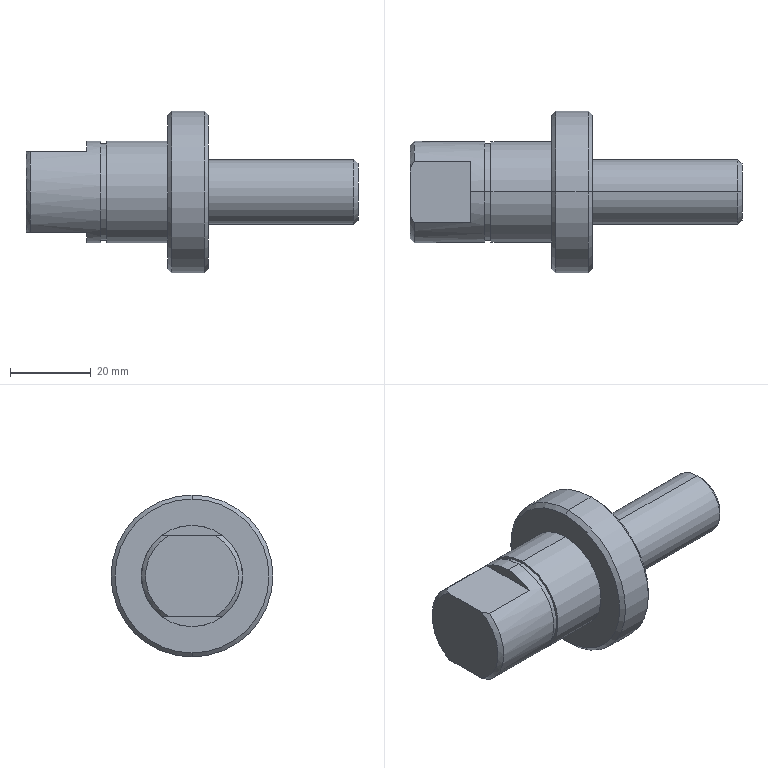Part | SolidWorks | features BaseBody 1 | 1 solid | 28 faces | box 82 x 40 x 40 mm | volume 36185 mm3 | cylinder 10 | plane 10 | cone 8 | commonest cylinder face diameters 25 x4 16 x2 23.9 x2 40 x2
STEP:
#1=CARTESIAN_POINT('',(-5.,0.,19.));
#2=VERTEX_POINT('',#1);
#3=CARTESIAN_POINT('',(-5.,0.,-19.));
#4=VERTEX_POINT('',#3);
#5=CARTESIAN_POINT('',(-5.,0.,0.));
#6=DIRECTION('',(-1.,0.,0.));
#7=DIRECTION('',(0.,0.,1.));
#8=AXIS2_PLACEMENT_3D('',#5,#6,#7);
#9=CIRCLE('',#8,19.);
#10=EDGE_CURVE('',#2,#4,#9,.T.);
#11=ORIENTED_EDGE('',*,*,#10,.F.);
#12=CARTESIAN_POINT('',(-4.,0.,20.));
#13=VERTEX_POINT('',#12);
#14=CARTESIAN_POINT('',(-4.,0.,20.));
#15=DIRECTION('',(0.7071,0.,0.7071));
#16=VECTOR('',#15,1000.);
#17=LINE('',#14,#16);
#18=EDGE_CURVE('',#2,#13,#17,.T.);
#19=ORIENTED_EDGE('',*,*,#18,.T.);
#20=CARTESIAN_POINT('',(-4.,0.,-20.));
#21=VERTEX_POINT('',#20);
#22=CARTESIAN_POINT('',(-4.,0.,0.));
#23=DIRECTION('',(1.,0.,0.));
#24=DIRECTION('',(0.,0.,1.));
#25=AXIS2_PLACEMENT_3D('',#22,#23,#24);
#26=CIRCLE('',#25,20.);
#27=EDGE_CURVE('',#21,#13,#26,.T.);
#28=ORIENTED_EDGE('',*,*,#27,.F.);
#29=CARTESIAN_POINT('',(-4.,0.,-20.));
#30=DIRECTION('',(0.7071,0.,-0.7071));
#31=VECTOR('',#30,1000.);
#32=LINE('',#29,#31);
#33=EDGE_CURVE('',#4,#21,#32,.T.);
#34=ORIENTED_EDGE('',*,*,#33,.F.);
#35=EDGE_LOOP('',(#11,#19,#28,#34));
#36=FACE_OUTER_BOUND('',#35,.T.);
#37=CARTESIAN_POINT('',(-4.,0.,0.));
#38=DIRECTION('',(1.,0.,0.));
#39=DIRECTION('',(0.,0.,-1.));
#40=AXIS2_PLACEMENT_3D('',#37,#38,#39);
#41=CONICAL_SURFACE('',#40,20.,0.7854);
#42=ADVANCED_FACE('',(#36),#41,.T.);
#43=CARTESIAN_POINT('',(5.,0.,-19.));
#44=VERTEX_POINT('',#43);
#45=CARTESIAN_POINT('',(5.,0.,19.));
#46=VERTEX_POINT('',#45);
#47=CARTESIAN_POINT('',(5.,0.,0.));
#48=DIRECTION('',(1.,0.,0.));
#49=DIRECTION('',(0.,0.,-1.));
#50=AXIS2_PLACEMENT_3D('',#47,#48,#49);
#51=CIRCLE('',#50,19.);
#52=EDGE_CURVE('',#44,#46,#51,.T.);
#53=ORIENTED_EDGE('',*,*,#52,.F.);
#54=CARTESIAN_POINT('',(4.,0.,-20.));
#55=VERTEX_POINT('',#54);
#56=CARTESIAN_POINT('',(5.,0.,-19.));
#57=DIRECTION('',(-0.7071,0.,-0.7071));
#58=VECTOR('',#57,1000.);
#59=LINE('',#56,#58);
#60=EDGE_CURVE('',#44,#55,#59,.T.);
#61=ORIENTED_EDGE('',*,*,#60,.T.);
#62=CARTESIAN_POINT('',(4.,0.,20.));
#63=VERTEX_POINT('',#62);
#64=CARTESIAN_POINT('',(4.,0.,0.));
#65=DIRECTION('',(-1.,0.,0.));
#66=DIRECTION('',(0.,0.,-1.));
#67=AXIS2_PLACEMENT_3D('',#64,#65,#66);
#68=CIRCLE('',#67,20.);
#69=EDGE_CURVE('',#63,#55,#68,.T.);
#70=ORIENTED_EDGE('',*,*,#69,.F.);
#71=CARTESIAN_POINT('',(5.,0.,19.));
#72=DIRECTION('',(-0.7071,0.,0.7071));
#73=VECTOR('',#72,1000.);
#74=LINE('',#71,#73);
#75=EDGE_CURVE('',#46,#63,#74,.T.);
#76=ORIENTED_EDGE('',*,*,#75,.F.);
#77=EDGE_LOOP('',(#53,#61,#70,#76));
#78=FACE_OUTER_BOUND('',#77,.T.);
#79=CARTESIAN_POINT('',(5.,0.,0.));
#80=DIRECTION('',(-1.,0.,0.));
#81=DIRECTION('',(0.,0.,1.));
#82=AXIS2_PLACEMENT_3D('',#79,#80,#81);
#83=CONICAL_SURFACE('',#82,19.,0.7854);
#84=ADVANCED_FACE('',(#78),#83,.T.);
#85=CARTESIAN_POINT('',(42.,0.,-7.));
#86=VERTEX_POINT('',#85);
#87=CARTESIAN_POINT('',(42.,0.,7.));
#88=VERTEX_POINT('',#87);
#89=CARTESIAN_POINT('',(42.,0.,0.));
#90=DIRECTION('',(1.,0.,0.));
#91=DIRECTION('',(0.,0.,-1.));
#92=AXIS2_PLACEMENT_3D('',#89,#90,#91);
#93=CIRCLE('',#92,7.);
#94=EDGE_CURVE('',#86,#88,#93,.T.);
#95=ORIENTED_EDGE('',*,*,#94,.F.);
#96=CARTESIAN_POINT('',(41.,0.,-8.));
#97=VERTEX_POINT('',#96);
#98=CARTESIAN_POINT('',(42.,0.,-7.));
#99=DIRECTION('',(-0.7071,0.,-0.7071));
#100=VECTOR('',#99,1000.);
#101=LINE('',#98,#100);
#102=EDGE_CURVE('',#86,#97,#101,.T.);
#103=ORIENTED_EDGE('',*,*,#102,.T.);
#104=CARTESIAN_POINT('',(41.,0.,8.));
#105=VERTEX_POINT('',#104);
#106=CARTESIAN_POINT('',(41.,0.,0.));
#107=DIRECTION('',(-1.,0.,0.));
#108=DIRECTION('',(0.,0.,-1.));
#109=AXIS2_PLACEMENT_3D('',#106,#107,#108);
#110=CIRCLE('',#109,8.);
#111=EDGE_CURVE('',#105,#97,#110,.T.);
#112=ORIENTED_EDGE('',*,*,#111,.F.);
#113=CARTESIAN_POINT('',(42.,0.,7.));
#114=DIRECTION('',(-0.7071,0.,0.7071));
#115=VECTOR('',#114,1000.);
#116=LINE('',#113,#115);
#117=EDGE_CURVE('',#88,#105,#116,.T.);
#118=ORIENTED_EDGE('',*,*,#117,.F.);
#119=EDGE_LOOP('',(#95,#103,#112,#118));
#120=FACE_OUTER_BOUND('',#119,.T.);
#121=CARTESIAN_POINT('',(42.,0.,0.));
#122=DIRECTION('',(-1.,0.,0.));
#123=DIRECTION('',(0.,0.,1.));
#124=AXIS2_PLACEMENT_3D('',#121,#122,#123);
#125=CONICAL_SURFACE('',#124,7.,0.7854);
#126=ADVANCED_FACE('',(#120),#125,.T.);
#127=CARTESIAN_POINT('',(-21.5,0.,-11.95));
#128=VERTEX_POINT('',#127);
#129=CARTESIAN_POINT('',(-21.5,0.,11.95));
#130=VERTEX_POINT('',#129);
#131=CARTESIAN_POINT('',(-21.5,0.,0.));
#132=DIRECTION('',(1.,0.,0.));
#133=DIRECTION('',(0.,0.,-1.));
#134=AXIS2_PLACEMENT_3D('',#131,#132,#133);
#135=CIRCLE('',#134,11.95);
#136=EDGE_CURVE('',#128,#130,#135,.T.);
#137=ORIENTED_EDGE('',*,*,#136,.T.);
#138=CARTESIAN_POINT('',(-20.,0.,11.95));
#139=VERTEX_POINT('',#138);
#140=CARTESIAN_POINT('',(0.,0.,11.95));
#141=DIRECTION('',(1.,0.,0.));
#142=VECTOR('',#141,1000.);
#143=LINE('',#140,#142);
#144=EDGE_CURVE('',#130,#139,#143,.T.);
#145=ORIENTED_EDGE('',*,*,#144,.T.);
#146=CARTESIAN_POINT('',(-20.,0.,-11.95));
#147=VERTEX_POINT('',#146);
#148=CARTESIAN_POINT('',(-20.,0.,0.));
#149=DIRECTION('',(1.,0.,0.));
#150=DIRECTION('',(0.,0.,-1.));
#151=AXIS2_PLACEMENT_3D('',#148,#149,#150);
#152=CIRCLE('',#151,11.95);
#153=EDGE_CURVE('',#147,#139,#152,.T.);
#154=ORIENTED_EDGE('',*,*,#153,.F.);
#155=CARTESIAN_POINT('',(0.,0.,-11.95));
#156=DIRECTION('',(1.,0.,0.));
#157=VECTOR('',#156,1000.);
#158=LINE('',#155,#157);
#159=EDGE_CURVE('',#128,#147,#158,.T.);
#160=ORIENTED_EDGE('',*,*,#159,.F.);
#161=EDGE_LOOP('',(#137,#145,#154,#160));
#162=FACE_OUTER_BOUND('',#161,.T.);
#163=CARTESIAN_POINT('',(0.,0.,0.));
#164=DIRECTION('',(1.,0.,0.));
#165=DIRECTION('',(0.,0.,-1.));
#166=AXIS2_PLACEMENT_3D('',#163,#164,#165);
#167=CYLINDRICAL_SURFACE('',#166,11.95);
#168=ADVANCED_FACE('',(#162),#167,.T.);
#169=CARTESIAN_POINT('',(-20.,0.,-12.5));
#170=VERTEX_POINT('',#169);
#171=CARTESIAN_POINT('',(-20.,0.,12.5));
#172=VERTEX_POINT('',#171);
#173=CARTESIAN_POINT('',(-20.,0.,0.));
#174=DIRECTION('',(1.,0.,0.));
#175=DIRECTION('',(0.,0.,-1.));
#176=AXIS2_PLACEMENT_3D('',#173,#174,#175);
#177=CIRCLE('',#176,12.5);
#178=EDGE_CURVE('',#170,#172,#177,.T.);
#179=ORIENTED_EDGE('',*,*,#178,.T.);
#180=CARTESIAN_POINT('',(-5.,0.,12.5));
#181=VERTEX_POINT('',#180);
#182=CARTESIAN_POINT('',(0.,0.,12.5));
#183=DIRECTION('',(1.,0.,0.));
#184=VECTOR('',#183,1000.);
#185=LINE('',#182,#184);
#186=EDGE_CURVE('',#172,#181,#185,.T.);
#187=ORIENTED_EDGE('',*,*,#186,.T.);
#188=CARTESIAN_POINT('',(-5.,0.,-12.5));
#189=VERTEX_POINT('',#188);
#190=CARTESIAN_POINT('',(-5.,0.,0.));
#191=DIRECTION('',(1.,0.,0.));
#192=DIRECTION('',(0.,0.,-1.));
#193=AXIS2_PLACEMENT_3D('',#190,#191,#192);
#194=CIRCLE('',#193,12.5);
#195=EDGE_CURVE('',#189,#181,#194,.T.);
#196=ORIENTED_EDGE('',*,*,#195,.F.);
#197=CARTESIAN_POINT('',(0.,0.,-12.5));
#198=DIRECTION('',(1.,0.,0.));
#199=VECTOR('',#198,1000.);
#200=LINE('',#197,#199);
#201=EDGE_CURVE('',#170,#189,#200,.T.);
#202=ORIENTED_EDGE('',*,*,#201,.F.);
#203=EDGE_LOOP('',(#179,#187,#196,#202));
#204=FACE_OUTER_BOUND('',#203,.T.);
#205=CARTESIAN_POINT('',(0.,0.,0.));
#206=DIRECTION('',(1.,0.,0.));
#207=DIRECTION('',(0.,0.,-1.));
#208=AXIS2_PLACEMENT_3D('',#205,#206,#207);
#209=CYLINDRICAL_SURFACE('',#208,12.5);
#210=ADVANCED_FACE('',(#204),#209,.T.);
#211=ORIENTED_EDGE('',*,*,#27,.T.);
#212=CARTESIAN_POINT('',(0.,0.,20.));
#213=DIRECTION('',(1.,0.,0.));
#214=VECTOR('',#213,1000.);
#215=LINE('',#212,#214);
#216=EDGE_CURVE('',#13,#63,#215,.T.);
#217=ORIENTED_EDGE('',*,*,#216,.T.);
#218=ORIENTED_EDGE('',*,*,#69,.T.);
#219=CARTESIAN_POINT('',(0.,0.,-20.));
#220=DIRECTION('',(1.,0.,0.));
#221=VECTOR('',#220,1000.);
#222=LINE('',#219,#221);
#223=EDGE_CURVE('',#21,#55,#222,.T.);
#224=ORIENTED_EDGE('',*,*,#223,.F.);
#225=EDGE_LOOP('',(#211,#217,#218,#224));
#226=FACE_OUTER_BOUND('',#225,.T.);
#227=CARTESIAN_POINT('',(0.,0.,0.));
#228=DIRECTION('',(1.,0.,0.));
#229=DIRECTION('',(0.,0.,-1.));
#230=AXIS2_PLACEMENT_3D('',#227,#228,#229);
#231=CYLINDRICAL_SURFACE('',#230,20.);
#232=ADVANCED_FACE('',(#226),#231,.T.);
#233=CARTESIAN_POINT('',(5.,0.,-8.));
#234=VERTEX_POINT('',#233);
#235=CARTESIAN_POINT('',(5.,0.,8.));
#236=VERTEX_POINT('',#235);
#237=CARTESIAN_POINT('',(5.,0.,0.));
#238=DIRECTION('',(1.,0.,0.));
#239=DIRECTION('',(0.,0.,-1.));
#240=AXIS2_PLACEMENT_3D('',#237,#238,#239);
#241=CIRCLE('',#240,8.);
#242=EDGE_CURVE('',#234,#236,#241,.T.);
#243=ORIENTED_EDGE('',*,*,#242,.T.);
#244=CARTESIAN_POINT('',(0.,0.,8.));
#245=DIRECTION('',(1.,0.,0.));
#246=VECTOR('',#245,1000.);
#247=LINE('',#244,#246);
#248=EDGE_CURVE('',#236,#105,#247,.T.);
#249=ORIENTED_EDGE('',*,*,#248,.T.);
#250=ORIENTED_EDGE('',*,*,#111,.T.);
#251=CARTESIAN_POINT('',(0.,0.,-8.));
#252=DIRECTION('',(1.,0.,0.));
#253=VECTOR('',#252,1000.);
#254=LINE('',#251,#253);
#255=EDGE_CURVE('',#234,#97,#254,.T.);
#256=ORIENTED_EDGE('',*,*,#255,.F.);
#257=EDGE_LOOP('',(#243,#249,#250,#256));
#258=FACE_OUTER_BOUND('',#257,.T.);
#259=CARTESIAN_POINT('',(0.,0.,0.));
#260=DIRECTION('',(1.,0.,0.));
#261=DIRECTION('',(0.,0.,-1.));
#262=AXIS2_PLACEMENT_3D('',#259,#260,#261);
#263=CYLINDRICAL_SURFACE('',#262,8.);
#264=ADVANCED_FACE('',(#258),#263,.T.);
#265=CARTESIAN_POINT('',(-25.,7.5,10.));
#266=VERTEX_POINT('',#265);
#267=CARTESIAN_POINT('',(-25.,0.,12.5));
#268=VERTEX_POINT('',#267);
#269=CARTESIAN_POINT('',(-25.,0.,0.));
#270=DIRECTION('',(1.,0.,0.));
#271=DIRECTION('',(0.,0.,1.));
#272=AXIS2_PLACEMENT_3D('',#269,#270,#271);
#273=CIRCLE('',#272,12.5);
#274=EDGE_CURVE('',#266,#268,#273,.T.);
#275=ORIENTED_EDGE('',*,*,#274,.T.);
#276=CARTESIAN_POINT('',(-21.5,0.,12.5));
#277=VERTEX_POINT('',#276);
#278=CARTESIAN_POINT('',(0.,0.,12.5));
#279=DIRECTION('',(1.,0.,0.));
#280=VECTOR('',#279,1000.);
#281=LINE('',#278,#280);
#282=EDGE_CURVE('',#268,#277,#281,.T.);
#283=ORIENTED_EDGE('',*,*,#282,.T.);
#284=CARTESIAN_POINT('',(-21.5,0.,-12.5));
#285=VERTEX_POINT('',#284);
#286=CARTESIAN_POINT('',(-21.5,0.,0.));
#287=DIRECTION('',(1.,0.,0.));
#288=DIRECTION('',(0.,0.,-1.));
#289=AXIS2_PLACEMENT_3D('',#286,#287,#288);
#290=CIRCLE('',#289,12.5);
#291=EDGE_CURVE('',#285,#277,#290,.T.);
#292=ORIENTED_EDGE('',*,*,#291,.F.);
#293=CARTESIAN_POINT('',(-25.,0.,-12.5));
#294=VERTEX_POINT('',#293);
#295=CARTESIAN_POINT('',(0.,0.,-12.5));
#296=DIRECTION('',(1.,0.,0.));
#297=VECTOR('',#296,1000.);
#298=LINE('',#295,#297);
#299=EDGE_CURVE('',#294,#285,#298,.T.);
#300=ORIENTED_EDGE('',*,*,#299,.F.);
#301=CARTESIAN_POINT('',(-25.,7.5,-10.));
#302=VERTEX_POINT('',#301);
#303=CARTESIAN_POINT('',(-25.,0.,0.));
#304=DIRECTION('',(1.,0.,0.));
#305=DIRECTION('',(0.,0.,1.));
#306=AXIS2_PLACEMENT_3D('',#303,#304,#305);
#307=CIRCLE('',#306,12.5);
#308=EDGE_CURVE('',#294,#302,#307,.T.);
#309=ORIENTED_EDGE('',*,*,#308,.T.);
#310=CARTESIAN_POINT('',(-39.,7.5,-10.));
#311=VERTEX_POINT('',#310);
#312=CARTESIAN_POINT('',(0.,7.5,-10.));
#313=DIRECTION('',(-1.,0.,0.));
#314=VECTOR('',#313,1000.);
#315=LINE('',#312,#314);
#316=EDGE_CURVE('',#302,#311,#315,.T.);
#317=ORIENTED_EDGE('',*,*,#316,.T.);
#318=CARTESIAN_POINT('',(-39.,7.5,10.));
#319=VERTEX_POINT('',#318);
#320=CARTESIAN_POINT('',(-39.,0.,0.));
#321=DIRECTION('',(1.,0.,0.));
#322=DIRECTION('',(0.,0.,1.));
#323=AXIS2_PLACEMENT_3D('',#320,#321,#322);
#324=CIRCLE('',#323,12.5);
#325=EDGE_CURVE('',#311,#319,#324,.T.);
#326=ORIENTED_EDGE('',*,*,#325,.T.);
#327=CARTESIAN_POINT('',(0.,7.5,10.));
#328=DIRECTION('',(1.,0.,0.));
#329=VECTOR('',#328,1000.);
#330=LINE('',#327,#329);
#331=EDGE_CURVE('',#319,#266,#330,.T.);
#332=ORIENTED_EDGE('',*,*,#331,.T.);
#333=EDGE_LOOP('',(#275,#283,#292,#300,#309,#317,#326,#332));
#334=FACE_OUTER_BOUND('',#333,.T.);
#335=CARTESIAN_POINT('',(0.,0.,0.));
#336=DIRECTION('',(1.,0.,0.));
#337=DIRECTION('',(0.,0.,-1.));
#338=AXIS2_PLACEMENT_3D('',#335,#336,#337);
#339=CYLINDRICAL_SURFACE('',#338,12.5);
#340=ADVANCED_FACE('',(#334),#339,.T.);
#341=ORIENTED_EDGE('',*,*,#282,.F.);
#342=CARTESIAN_POINT('',(-25.,-7.5,10.));
#343=VERTEX_POINT('',#342);
#344=CARTESIAN_POINT('',(-25.,0.,0.));
#345=DIRECTION('',(1.,0.,0.));
#346=DIRECTION('',(0.,0.,1.));
#347=AXIS2_PLACEMENT_3D('',#344,#345,#346);
#348=CIRCLE('',#347,12.5);
#349=EDGE_CURVE('',#268,#343,#348,.T.);
#350=ORIENTED_EDGE('',*,*,#349,.T.);
#351=CARTESIAN_POINT('',(-39.,-7.5,10.));
#352=VERTEX_POINT('',#351);
#353=CARTESIAN_POINT('',(0.,-7.5,10.));
#354=DIRECTION('',(-1.,0.,0.));
#355=VECTOR('',#354,1000.);
#356=LINE('',#353,#355);
#357=EDGE_CURVE('',#343,#352,#356,.T.);
#358=ORIENTED_EDGE('',*,*,#357,.T.);
#359=CARTESIAN_POINT('',(-39.,-7.5,-10.));
#360=VERTEX_POINT('',#359);
#361=CARTESIAN_POINT('',(-39.,0.,0.));
#362=DIRECTION('',(1.,0.,0.));
#363=DIRECTION('',(0.,0.,1.));
#364=AXIS2_PLACEMENT_3D('',#361,#362,#363);
#365=CIRCLE('',#364,12.5);
#366=EDGE_CURVE('',#352,#360,#365,.T.);
#367=ORIENTED_EDGE('',*,*,#366,.T.);
#368=CARTESIAN_POINT('',(-25.,-7.5,-10.));
#369=VERTEX_POINT('',#368);
#370=CARTESIAN_POINT('',(0.,-7.5,-10.));
#371=DIRECTION('',(1.,0.,0.));
#372=VECTOR('',#371,1000.);
#373=LINE('',#370,#372);
#374=EDGE_CURVE('',#360,#369,#373,.T.);
#375=ORIENTED_EDGE('',*,*,#374,.T.);
#376=CARTESIAN_POINT('',(-25.,0.,0.));
#377=DIRECTION('',(1.,0.,0.));
#378=DIRECTION('',(0.,0.,1.));
#379=AXIS2_PLACEMENT_3D('',#376,#377,#378);
#380=CIRCLE('',#379,12.5);
#381=EDGE_CURVE('',#369,#294,#380,.T.);
#382=ORIENTED_EDGE('',*,*,#381,.T.);
#383=ORIENTED_EDGE('',*,*,#299,.T.);
#384=CARTESIAN_POINT('',(-21.5,0.,0.));
#385=DIRECTION('',(1.,0.,0.));
#386=DIRECTION('',(0.,0.,-1.));
#387=AXIS2_PLACEMENT_3D('',#384,#385,#386);
#388=CIRCLE('',#387,12.5);
#389=EDGE_CURVE('',#277,#285,#388,.T.);
#390=ORIENTED_EDGE('',*,*,#389,.F.);
#391=EDGE_LOOP('',(#341,#350,#358,#367,#375,#382,#383,#390));
#392=FACE_OUTER_BOUND('',#391,.T.);
#393=CARTESIAN_POINT('',(0.,0.,0.));
#394=DIRECTION('',(1.,0.,0.));
#395=DIRECTION('',(0.,0.,-1.));
#396=AXIS2_PLACEMENT_3D('',#393,#394,#395);
#397=CYLINDRICAL_SURFACE('',#396,12.5);
#398=ADVANCED_FACE('',(#392),#397,.T.);
#399=CARTESIAN_POINT('',(-40.,-5.679,-10.));
#400=VERTEX_POINT('',#399);
#401=CARTESIAN_POINT('',(-40.,-5.679,10.));
#402=VERTEX_POINT('',#401);
#403=CARTESIAN_POINT('',(-40.,0.,0.));
#404=DIRECTION('',(-1.,0.,0.));
#405=DIRECTION('',(0.,0.,1.));
#406=AXIS2_PLACEMENT_3D('',#403,#404,#405);
#407=CIRCLE('',#406,11.5);
#408=EDGE_CURVE('',#400,#402,#407,.T.);
#409=ORIENTED_EDGE('',*,*,#408,.T.);
#410=CARTESIAN_POINT('',(-40.,5.679,10.));
#411=VERTEX_POINT('',#410);
#412=CARTESIAN_POINT('',(-40.,-15.,10.));
#413=DIRECTION('',(0.,1.,0.));
#414=VECTOR('',#413,1000.);
#415=LINE('',#412,#414);
#416=EDGE_CURVE('',#402,#411,#415,.T.);
#417=ORIENTED_EDGE('',*,*,#416,.T.);
#418=CARTESIAN_POINT('',(-40.,5.679,-10.));
#419=VERTEX_POINT('',#418);
#420=CARTESIAN_POINT('',(-40.,0.,0.));
#421=DIRECTION('',(-1.,0.,0.));
#422=DIRECTION('',(0.,0.,1.));
#423=AXIS2_PLACEMENT_3D('',#420,#421,#422);
#424=CIRCLE('',#423,11.5);
#425=EDGE_CURVE('',#411,#419,#424,.T.);
#426=ORIENTED_EDGE('',*,*,#425,.T.);
#427=CARTESIAN_POINT('',(-40.,-15.,-10.));
#428=DIRECTION('',(0.,-1.,0.));
#429=VECTOR('',#428,1000.);
#430=LINE('',#427,#429);
#431=EDGE_CURVE('',#419,#400,#430,.T.);
#432=ORIENTED_EDGE('',*,*,#431,.T.);
#433=EDGE_LOOP('',(#409,#417,#426,#432));
#434=FACE_OUTER_BOUND('',#433,.T.);
#435=CARTESIAN_POINT('',(-40.,12.5,0.));
#436=DIRECTION('',(-1.,0.,0.));
#437=DIRECTION('',(0.,0.,1.));
#438=AXIS2_PLACEMENT_3D('',#435,#436,#437);
#439=PLANE('',#438);
#440=ADVANCED_FACE('',(#434),#439,.T.);
#441=ORIENTED_EDGE('',*,*,#366,.F.);
#442=CARTESIAN_POINT('',(-39.,-7.5,10.));
#443=CARTESIAN_POINT('',(-39.357,-6.905,10.));
#444=CARTESIAN_POINT('',(-39.694,-6.299,10.));
#445=CARTESIAN_POINT('',(-40.,-5.679,10.));
#446=B_SPLINE_CURVE_WITH_KNOTS('',3,(#442,#443,#444,#445),.UNSPECIFIED.,.F.,.F.,(4,4),(0.02358,0.02565),.UNSPECIFIED.);
#447=EDGE_CURVE('',#352,#402,#446,.T.);
#448=ORIENTED_EDGE('',*,*,#447,.T.);
#449=ORIENTED_EDGE('',*,*,#408,.F.);
#450=CARTESIAN_POINT('',(-40.,-5.679,-10.));
#451=CARTESIAN_POINT('',(-39.693,-6.301,-10.));
#452=CARTESIAN_POINT('',(-39.356,-6.906,-10.));
#453=CARTESIAN_POINT('',(-39.,-7.5,-10.));
#454=B_SPLINE_CURVE_WITH_KNOTS('',3,(#450,#451,#452,#453),.UNSPECIFIED.,.F.,.F.,(4,4),(0.03752,0.03962),.UNSPECIFIED.);
#455=EDGE_CURVE('',#400,#360,#454,.T.);
#456=ORIENTED_EDGE('',*,*,#455,.T.);
#457=EDGE_LOOP('',(#441,#448,#449,#456));
#458=FACE_OUTER_BOUND('',#457,.T.);
#459=CARTESIAN_POINT('',(-39.,0.,0.));
#460=DIRECTION('',(1.,0.,0.));
#461=DIRECTION('',(0.,0.,-1.));
#462=AXIS2_PLACEMENT_3D('',#459,#460,#461);
#463=CONICAL_SURFACE('',#462,12.5,0.7854);
#464=ADVANCED_FACE('',(#458),#463,.T.);
#465=ORIENTED_EDGE('',*,*,#425,.F.);
#466=CARTESIAN_POINT('',(-40.,5.679,10.));
#467=CARTESIAN_POINT('',(-39.693,6.301,10.));
#468=CARTESIAN_POINT('',(-39.356,6.906,10.));
#469=CARTESIAN_POINT('',(-39.,7.5,10.));
#470=B_SPLINE_CURVE_WITH_KNOTS('',3,(#466,#467,#468,#469),.UNSPECIFIED.,.F.,.F.,(4,4),(0.03752,0.03962),.UNSPECIFIED.);
#471=EDGE_CURVE('',#411,#319,#470,.T.);
#472=ORIENTED_EDGE('',*,*,#471,.T.);
#473=ORIENTED_EDGE('',*,*,#325,.F.);
#474=CARTESIAN_POINT('',(-39.,7.5,-10.));
#475=CARTESIAN_POINT('',(-39.357,6.905,-10.));
#476=CARTESIAN_POINT('',(-39.694,6.299,-10.));
#477=CARTESIAN_POINT('',(-40.,5.679,-10.));
#478=B_SPLINE_CURVE_WITH_KNOTS('',3,(#474,#475,#476,#477),.UNSPECIFIED.,.F.,.F.,(4,4),(0.02358,0.02565),.UNSPECIFIED.);
#479=EDGE_CURVE('',#311,#419,#478,.T.);
#480=ORIENTED_EDGE('',*,*,#479,.T.);
#481=EDGE_LOOP('',(#465,#472,#473,#480));
#482=FACE_OUTER_BOUND('',#481,.T.);
#483=CARTESIAN_POINT('',(-39.,0.,0.));
#484=DIRECTION('',(1.,0.,0.));
#485=DIRECTION('',(0.,0.,-1.));
#486=AXIS2_PLACEMENT_3D('',#483,#484,#485);
#487=CONICAL_SURFACE('',#486,12.5,0.7854);
#488=ADVANCED_FACE('',(#482),#487,.T.);
#489=CARTESIAN_POINT('',(42.,0.,0.));
#490=DIRECTION('',(1.,0.,0.));
#491=DIRECTION('',(0.,0.,-1.));
#492=AXIS2_PLACEMENT_3D('',#489,#490,#491);
#493=CIRCLE('',#492,7.);
#494=EDGE_CURVE('',#88,#86,#493,.T.);
#495=ORIENTED_EDGE('',*,*,#494,.T.);
#496=ORIENTED_EDGE('',*,*,#94,.T.);
#497=EDGE_LOOP('',(#495,#496));
#498=FACE_OUTER_BOUND('',#497,.T.);
#499=CARTESIAN_POINT('',(42.,0.,0.));
#500=DIRECTION('',(1.,0.,0.));
#501=DIRECTION('',(0.,0.,-1.));
#502=AXIS2_PLACEMENT_3D('',#499,#500,#501);
#503=PLANE('',#502);
#504=ADVANCED_FACE('',(#498),#503,.T.);
#505=ORIENTED_EDGE('',*,*,#248,.F.);
#506=CARTESIAN_POINT('',(5.,0.,0.));
#507=DIRECTION('',(1.,0.,0.));
#508=DIRECTION('',(0.,0.,-1.));
#509=AXIS2_PLACEMENT_3D('',#506,#507,#508);
#510=CIRCLE('',#509,8.);
#511=EDGE_CURVE('',#236,#234,#510,.T.);
#512=ORIENTED_EDGE('',*,*,#511,.T.);
#513=ORIENTED_EDGE('',*,*,#255,.T.);
#514=CARTESIAN_POINT('',(41.,0.,0.));
#515=DIRECTION('',(-1.,0.,0.));
#516=DIRECTION('',(0.,0.,-1.));
#517=AXIS2_PLACEMENT_3D('',#514,#515,#516);
#518=CIRCLE('',#517,8.);
#519=EDGE_CURVE('',#97,#105,#518,.T.);
#520=ORIENTED_EDGE('',*,*,#519,.T.);
#521=EDGE_LOOP('',(#505,#512,#513,#520));
#522=FACE_OUTER_BOUND('',#521,.T.);
#523=CARTESIAN_POINT('',(0.,0.,0.));
#524=DIRECTION('',(1.,0.,0.));
#525=DIRECTION('',(0.,0.,-1.));
#526=AXIS2_PLACEMENT_3D('',#523,#524,#525);
#527=CYLINDRICAL_SURFACE('',#526,8.);
#528=ADVANCED_FACE('',(#522),#527,.T.);
#529=CARTESIAN_POINT('',(5.,0.,0.));
#530=DIRECTION('',(1.,0.,0.));
#531=DIRECTION('',(0.,0.,-1.));
#532=AXIS2_PLACEMENT_3D('',#529,#530,#531);
#533=CIRCLE('',#532,19.);
#534=EDGE_CURVE('',#46,#44,#533,.T.);
#535=ORIENTED_EDGE('',*,*,#534,.T.);
#536=ORIENTED_EDGE('',*,*,#52,.T.);
#537=EDGE_LOOP('',(#535,#536));
#538=FACE_OUTER_BOUND('',#537,.T.);
#539=ORIENTED_EDGE('',*,*,#242,.F.);
#540=ORIENTED_EDGE('',*,*,#511,.F.);
#541=EDGE_LOOP('',(#539,#540));
#542=FACE_BOUND('',#541,.T.);
#543=CARTESIAN_POINT('',(5.,8.,0.));
#544=DIRECTION('',(1.,0.,0.));
#545=DIRECTION('',(0.,0.,-1.));
#546=AXIS2_PLACEMENT_3D('',#543,#544,#545);
#547=PLANE('',#546);
#548=ADVANCED_FACE('',(#538,#542),#547,.T.);
#549=ORIENTED_EDGE('',*,*,#216,.F.);
#550=CARTESIAN_POINT('',(-4.,0.,0.));
#551=DIRECTION('',(1.,0.,0.));
#552=DIRECTION('',(0.,0.,1.));
#553=AXIS2_PLACEMENT_3D('',#550,#551,#552);
#554=CIRCLE('',#553,20.);
#555=EDGE_CURVE('',#13,#21,#554,.T.);
#556=ORIENTED_EDGE('',*,*,#555,.T.);
#557=ORIENTED_EDGE('',*,*,#223,.T.);
#558=CARTESIAN_POINT('',(4.,0.,0.));
#559=DIRECTION('',(-1.,0.,0.));
#560=DIRECTION('',(0.,0.,-1.));
#561=AXIS2_PLACEMENT_3D('',#558,#559,#560);
#562=CIRCLE('',#561,20.);
#563=EDGE_CURVE('',#55,#63,#562,.T.);
#564=ORIENTED_EDGE('',*,*,#563,.T.);
#565=EDGE_LOOP('',(#549,#556,#557,#564));
#566=FACE_OUTER_BOUND('',#565,.T.);
#567=CARTESIAN_POINT('',(0.,0.,0.));
#568=DIRECTION('',(1.,0.,0.));
#569=DIRECTION('',(0.,0.,-1.));
#570=AXIS2_PLACEMENT_3D('',#567,#568,#569);
#571=CYLINDRICAL_SURFACE('',#570,20.);
#572=ADVANCED_FACE('',(#566),#571,.T.);
#573=CARTESIAN_POINT('',(-5.,0.,0.));
#574=DIRECTION('',(-1.,0.,0.));
#575=DIRECTION('',(0.,0.,1.));
#576=AXIS2_PLACEMENT_3D('',#573,#574,#575);
#577=CIRCLE('',#576,19.);
#578=EDGE_CURVE('',#4,#2,#577,.T.);
#579=ORIENTED_EDGE('',*,*,#578,.T.);
#580=ORIENTED_EDGE('',*,*,#10,.T.);
#581=EDGE_LOOP('',(#579,#580));
#582=FACE_OUTER_BOUND('',#581,.T.);
#583=ORIENTED_EDGE('',*,*,#195,.T.);
#584=CARTESIAN_POINT('',(-5.,0.,0.));
#585=DIRECTION('',(1.,0.,0.));
#586=DIRECTION('',(0.,0.,-1.));
#587=AXIS2_PLACEMENT_3D('',#584,#585,#586);
#588=CIRCLE('',#587,12.5);
#589=EDGE_CURVE('',#181,#189,#588,.T.);
#590=ORIENTED_EDGE('',*,*,#589,.T.);
#591=EDGE_LOOP('',(#583,#590));
#592=FACE_BOUND('',#591,.T.);
#593=CARTESIAN_POINT('',(-5.,20.,0.));
#594=DIRECTION('',(-1.,0.,0.));
#595=DIRECTION('',(0.,0.,1.));
#596=AXIS2_PLACEMENT_3D('',#593,#594,#595);
#597=PLANE('',#596);
#598=ADVANCED_FACE('',(#582,#592),#597,.T.);
#599=ORIENTED_EDGE('',*,*,#186,.F.);
#600=CARTESIAN_POINT('',(-20.,0.,0.));
#601=DIRECTION('',(1.,0.,0.));
#602=DIRECTION('',(0.,0.,-1.));
#603=AXIS2_PLACEMENT_3D('',#600,#601,#602);
#604=CIRCLE('',#603,12.5);
#605=EDGE_CURVE('',#172,#170,#604,.T.);
#606=ORIENTED_EDGE('',*,*,#605,.T.);
#607=ORIENTED_EDGE('',*,*,#201,.T.);
#608=ORIENTED_EDGE('',*,*,#589,.F.);
#609=EDGE_LOOP('',(#599,#606,#607,#608));
#610=FACE_OUTER_BOUND('',#609,.T.);
#611=CARTESIAN_POINT('',(0.,0.,0.));
#612=DIRECTION('',(1.,0.,0.));
#613=DIRECTION('',(0.,0.,-1.));
#614=AXIS2_PLACEMENT_3D('',#611,#612,#613);
#615=CYLINDRICAL_SURFACE('',#614,12.5);
#616=ADVANCED_FACE('',(#610),#615,.T.);
#617=ORIENTED_EDGE('',*,*,#153,.T.);
#618=CARTESIAN_POINT('',(-20.,0.,0.));
#619=DIRECTION('',(1.,0.,0.));
#620=DIRECTION('',(0.,0.,-1.));
#621=AXIS2_PLACEMENT_3D('',#618,#619,#620);
#622=CIRCLE('',#621,11.95);
#623=EDGE_CURVE('',#139,#147,#622,.T.);
#624=ORIENTED_EDGE('',*,*,#623,.T.);
#625=EDGE_LOOP('',(#617,#624));
#626=FACE_BOUND('',#625,.T.);
#627=ORIENTED_EDGE('',*,*,#178,.F.);
#628=ORIENTED_EDGE('',*,*,#605,.F.);
#629=EDGE_LOOP('',(#627,#628));
#630=FACE_OUTER_BOUND('',#629,.T.);
#631=CARTESIAN_POINT('',(-20.,12.5,0.));
#632=DIRECTION('',(-1.,0.,0.));
#633=DIRECTION('',(0.,0.,1.));
#634=AXIS2_PLACEMENT_3D('',#631,#632,#633);
#635=PLANE('',#634);
#636=ADVANCED_FACE('',(#626,#630),#635,.T.);
#637=ORIENTED_EDGE('',*,*,#144,.F.);
#638=CARTESIAN_POINT('',(-21.5,0.,0.));
#639=DIRECTION('',(1.,0.,0.));
#640=DIRECTION('',(0.,0.,-1.));
#641=AXIS2_PLACEMENT_3D('',#638,#639,#640);
#642=CIRCLE('',#641,11.95);
#643=EDGE_CURVE('',#130,#128,#642,.T.);
#644=ORIENTED_EDGE('',*,*,#643,.T.);
#645=ORIENTED_EDGE('',*,*,#159,.T.);
#646=ORIENTED_EDGE('',*,*,#623,.F.);
#647=EDGE_LOOP('',(#637,#644,#645,#646));
#648=FACE_OUTER_BOUND('',#647,.T.);
#649=CARTESIAN_POINT('',(0.,0.,0.));
#650=DIRECTION('',(1.,0.,0.));
#651=DIRECTION('',(0.,0.,-1.));
#652=AXIS2_PLACEMENT_3D('',#649,#650,#651);
#653=CYLINDRICAL_SURFACE('',#652,11.95);
#654=ADVANCED_FACE('',(#648),#653,.T.);
#655=ORIENTED_EDGE('',*,*,#291,.T.);
#656=ORIENTED_EDGE('',*,*,#389,.T.);
#657=EDGE_LOOP('',(#655,#656));
#658=FACE_OUTER_BOUND('',#657,.T.);
#659=ORIENTED_EDGE('',*,*,#136,.F.);
#660=ORIENTED_EDGE('',*,*,#643,.F.);
#661=EDGE_LOOP('',(#659,#660));
#662=FACE_BOUND('',#661,.T.);
#663=CARTESIAN_POINT('',(-21.5,11.95,0.));
#664=DIRECTION('',(1.,0.,0.));
#665=DIRECTION('',(0.,0.,-1.));
#666=AXIS2_PLACEMENT_3D('',#663,#664,#665);
#667=PLANE('',#666);
#668=ADVANCED_FACE('',(#658,#662),#667,.T.);
#669=ORIENTED_EDGE('',*,*,#102,.F.);
#670=ORIENTED_EDGE('',*,*,#494,.F.);
#671=ORIENTED_EDGE('',*,*,#117,.T.);
#672=ORIENTED_EDGE('',*,*,#519,.F.);
#673=EDGE_LOOP('',(#669,#670,#671,#672));
#674=FACE_OUTER_BOUND('',#673,.T.);
#675=CARTESIAN_POINT('',(42.,0.,0.));
#676=DIRECTION('',(-1.,0.,0.));
#677=DIRECTION('',(0.,0.,1.));
#678=AXIS2_PLACEMENT_3D('',#675,#676,#677);
#679=CONICAL_SURFACE('',#678,7.,0.7854);
#680=ADVANCED_FACE('',(#674),#679,.T.);
#681=ORIENTED_EDGE('',*,*,#60,.F.);
#682=ORIENTED_EDGE('',*,*,#534,.F.);
#683=ORIENTED_EDGE('',*,*,#75,.T.);
#684=ORIENTED_EDGE('',*,*,#563,.F.);
#685=EDGE_LOOP('',(#681,#682,#683,#684));
#686=FACE_OUTER_BOUND('',#685,.T.);
#687=CARTESIAN_POINT('',(5.,0.,0.));
#688=DIRECTION('',(-1.,0.,0.));
#689=DIRECTION('',(0.,0.,1.));
#690=AXIS2_PLACEMENT_3D('',#687,#688,#689);
#691=CONICAL_SURFACE('',#690,19.,0.7854);
#692=ADVANCED_FACE('',(#686),#691,.T.);
#693=ORIENTED_EDGE('',*,*,#18,.F.);
#694=ORIENTED_EDGE('',*,*,#578,.F.);
#695=ORIENTED_EDGE('',*,*,#33,.T.);
#696=ORIENTED_EDGE('',*,*,#555,.F.);
#697=EDGE_LOOP('',(#693,#694,#695,#696));
#698=FACE_OUTER_BOUND('',#697,.T.);
#699=CARTESIAN_POINT('',(-4.,0.,0.));
#700=DIRECTION('',(1.,0.,0.));
#701=DIRECTION('',(0.,0.,-1.));
#702=AXIS2_PLACEMENT_3D('',#699,#700,#701);
#703=CONICAL_SURFACE('',#702,20.,0.7854);
#704=ADVANCED_FACE('',(#698),#703,.T.);
#705=CARTESIAN_POINT('',(-25.,-15.,-10.));
#706=DIRECTION('',(0.,-1.,0.));
#707=VECTOR('',#706,1000.);
#708=LINE('',#705,#707);
#709=EDGE_CURVE('',#302,#369,#708,.T.);
#710=ORIENTED_EDGE('',*,*,#709,.T.);
#711=ORIENTED_EDGE('',*,*,#374,.F.);
#712=ORIENTED_EDGE('',*,*,#455,.F.);
#713=ORIENTED_EDGE('',*,*,#431,.F.);
#714=ORIENTED_EDGE('',*,*,#479,.F.);
#715=ORIENTED_EDGE('',*,*,#316,.F.);
#716=EDGE_LOOP('',(#710,#711,#712,#713,#714,#715));
#717=FACE_OUTER_BOUND('',#716,.T.);
#718=CARTESIAN_POINT('',(-25.,-15.,-10.));
#719=DIRECTION('',(0.,0.,-1.));
#720=DIRECTION('',(-1.,0.,0.));
#721=AXIS2_PLACEMENT_3D('',#718,#719,#720);
#722=PLANE('',#721);
#723=ADVANCED_FACE('',(#717),#722,.T.);
#724=ORIENTED_EDGE('',*,*,#709,.F.);
#725=ORIENTED_EDGE('',*,*,#308,.F.);
#726=ORIENTED_EDGE('',*,*,#381,.F.);
#727=EDGE_LOOP('',(#724,#725,#726));
#728=FACE_OUTER_BOUND('',#727,.T.);
#729=CARTESIAN_POINT('',(-25.,0.,0.));
#730=DIRECTION('',(-1.,0.,0.));
#731=DIRECTION('',(0.,0.,1.));
#732=AXIS2_PLACEMENT_3D('',#729,#730,#731);
#733=PLANE('',#732);
#734=ADVANCED_FACE('',(#728),#733,.T.);
#735=CARTESIAN_POINT('',(-25.,-15.,10.));
#736=DIRECTION('',(0.,1.,0.));
#737=VECTOR('',#736,1000.);
#738=LINE('',#735,#737);
#739=EDGE_CURVE('',#343,#266,#738,.T.);
#740=ORIENTED_EDGE('',*,*,#739,.F.);
#741=ORIENTED_EDGE('',*,*,#349,.F.);
#742=ORIENTED_EDGE('',*,*,#274,.F.);
#743=EDGE_LOOP('',(#740,#741,#742));
#744=FACE_OUTER_BOUND('',#743,.T.);
#745=CARTESIAN_POINT('',(-25.,0.,0.));
#746=DIRECTION('',(-1.,0.,0.));
#747=DIRECTION('',(0.,0.,1.));
#748=AXIS2_PLACEMENT_3D('',#745,#746,#747);
#749=PLANE('',#748);
#750=ADVANCED_FACE('',(#744),#749,.T.);
#751=ORIENTED_EDGE('',*,*,#739,.T.);
#752=ORIENTED_EDGE('',*,*,#331,.F.);
#753=ORIENTED_EDGE('',*,*,#471,.F.);
#754=ORIENTED_EDGE('',*,*,#416,.F.);
#755=ORIENTED_EDGE('',*,*,#447,.F.);
#756=ORIENTED_EDGE('',*,*,#357,.F.);
#757=EDGE_LOOP('',(#751,#752,#753,#754,#755,#756));
#758=FACE_OUTER_BOUND('',#757,.T.);
#759=CARTESIAN_POINT('',(-25.,-15.,10.));
#760=DIRECTION('',(0.,0.,1.));
#761=DIRECTION('',(1.,0.,0.));
#762=AXIS2_PLACEMENT_3D('',#759,#760,#761);
#763=PLANE('',#762);
#764=ADVANCED_FACE('',(#758),#763,.T.);
#765=CLOSED_SHELL('',(#42,#84,#126,#168,#210,#232,#264,#340,#398,#440,#464,#488,#504,#528,#548,#572,#598,#616,#636,#654,#668,#680,#692,#704,#723,#734,#750,#764));
#766=MANIFOLD_SOLID_BREP('',#765);
#767=CARTESIAN_POINT('',(0.,0.,0.));
#768=DIRECTION('',(0.,0.,1.));
#769=DIRECTION('',(1.,0.,0.));
#770=AXIS2_PLACEMENT_3D('',#767,#768,#769);
#771=(LENGTH_UNIT()NAMED_UNIT(*)SI_UNIT(.MILLI.,.METRE.));
#772=UNCERTAINTY_MEASURE_WITH_UNIT(LENGTH_MEASURE(0.00001),#771,'','');
#773=(NAMED_UNIT(*)PLANE_ANGLE_UNIT()SI_UNIT($,.RADIAN.));
#774=(NAMED_UNIT(*)SI_UNIT($,.STERADIAN.)SOLID_ANGLE_UNIT());
#775=(GEOMETRIC_REPRESENTATION_CONTEXT(3)GLOBAL_UNCERTAINTY_ASSIGNED_CONTEXT((#772))GLOBAL_UNIT_ASSIGNED_CONTEXT((#771,#773,#774))REPRESENTATION_CONTEXT('',''));
#776=ADVANCED_BREP_SHAPE_REPRESENTATION('',(#766,#770),#775);